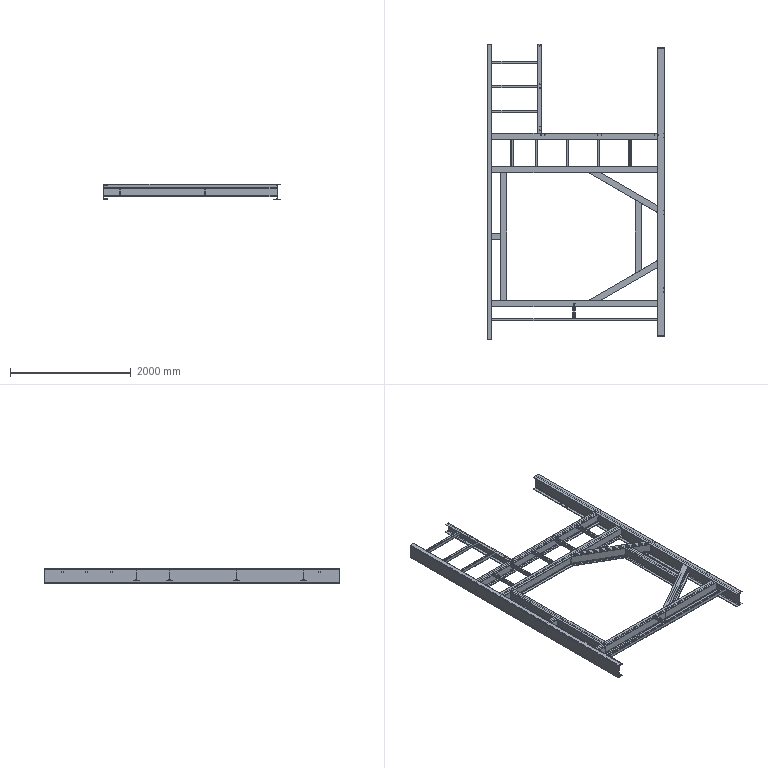Part | STEP file | PN_0025 third-floor left platform 1_Default<As Machined> | 21 solids | 573 faces | box 2948 x 4889 x 250 mm | volume 85593923 mm3 | plane 385 | cylinder 186 | cone 2 | commonest cylinder face diameters 26 x57 12 x42 6 x40 6.8 x19 10 x8 20 x8